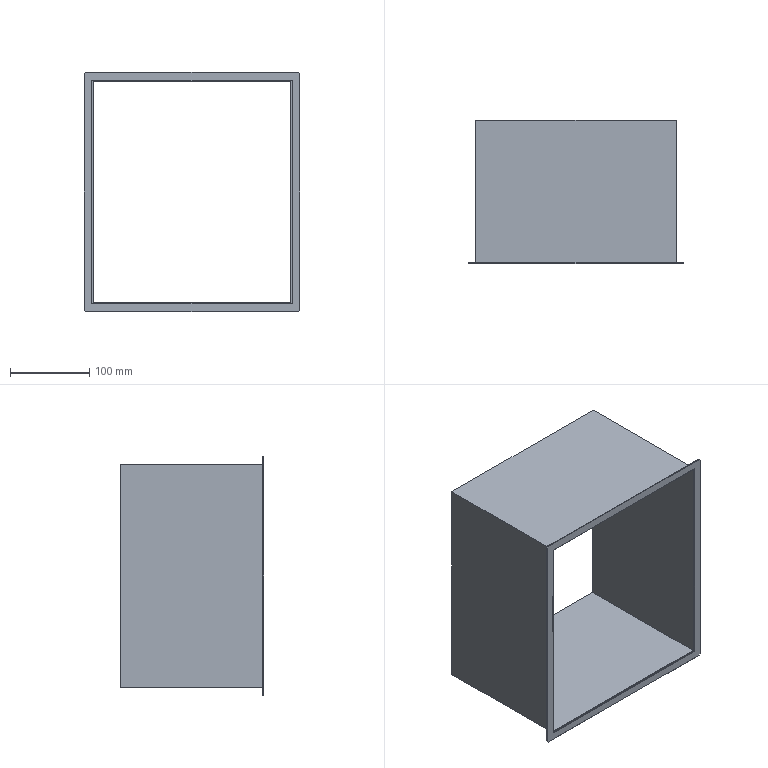Part | SolidWorks | features Chamfer 1, ExtruThin 1, ICE 1 | 2 solids | 24 faces | box 273 x 181.2 x 303 mm | volume 301154 mm3 | plane 24
STEP:
#1=CARTESIAN_POINT('',(126.5,180.,141.5));
#2=VERTEX_POINT('',#1);
#3=CARTESIAN_POINT('',(126.5,180.,-141.5));
#4=VERTEX_POINT('',#3);
#5=CARTESIAN_POINT('',(126.5,180.,0.));
#6=DIRECTION('',(0.,0.,-1.));
#7=VECTOR('',#6,1000.);
#8=LINE('',#5,#7);
#9=EDGE_CURVE('',#2,#4,#8,.T.);
#10=ORIENTED_EDGE('',*,*,#9,.T.);
#11=CARTESIAN_POINT('',(-126.5,180.,-141.5));
#12=VERTEX_POINT('',#11);
#13=CARTESIAN_POINT('',(0.,180.,-141.5));
#14=DIRECTION('',(-1.,0.,0.));
#15=VECTOR('',#14,1000.);
#16=LINE('',#13,#15);
#17=EDGE_CURVE('',#4,#12,#16,.T.);
#18=ORIENTED_EDGE('',*,*,#17,.T.);
#19=CARTESIAN_POINT('',(-126.5,180.,141.5));
#20=VERTEX_POINT('',#19);
#21=CARTESIAN_POINT('',(-126.5,180.,0.));
#22=DIRECTION('',(0.,0.,1.));
#23=VECTOR('',#22,1000.);
#24=LINE('',#21,#23);
#25=EDGE_CURVE('',#12,#20,#24,.T.);
#26=ORIENTED_EDGE('',*,*,#25,.T.);
#27=CARTESIAN_POINT('',(0.,180.,141.5));
#28=DIRECTION('',(1.,0.,0.));
#29=VECTOR('',#28,1000.);
#30=LINE('',#27,#29);
#31=EDGE_CURVE('',#20,#2,#30,.T.);
#32=ORIENTED_EDGE('',*,*,#31,.T.);
#33=EDGE_LOOP('',(#10,#18,#26,#32));
#34=FACE_OUTER_BOUND('',#33,.T.);
#35=CARTESIAN_POINT('',(125.,180.,-140.));
#36=VERTEX_POINT('',#35);
#37=CARTESIAN_POINT('',(-125.,180.,-140.));
#38=VERTEX_POINT('',#37);
#39=CARTESIAN_POINT('',(-125.,180.,-140.));
#40=DIRECTION('',(-1.,0.,0.));
#41=VECTOR('',#40,1000.);
#42=LINE('',#39,#41);
#43=EDGE_CURVE('',#36,#38,#42,.T.);
#44=ORIENTED_EDGE('',*,*,#43,.F.);
#45=CARTESIAN_POINT('',(125.,180.,140.));
#46=VERTEX_POINT('',#45);
#47=CARTESIAN_POINT('',(125.,180.,140.));
#48=DIRECTION('',(0.,0.,-1.));
#49=VECTOR('',#48,1000.);
#50=LINE('',#47,#49);
#51=EDGE_CURVE('',#46,#36,#50,.T.);
#52=ORIENTED_EDGE('',*,*,#51,.F.);
#53=CARTESIAN_POINT('',(-125.,180.,140.));
#54=VERTEX_POINT('',#53);
#55=CARTESIAN_POINT('',(-125.,180.,140.));
#56=DIRECTION('',(1.,0.,0.));
#57=VECTOR('',#56,1000.);
#58=LINE('',#55,#57);
#59=EDGE_CURVE('',#54,#46,#58,.T.);
#60=ORIENTED_EDGE('',*,*,#59,.F.);
#61=CARTESIAN_POINT('',(-125.,180.,140.));
#62=DIRECTION('',(0.,0.,1.));
#63=VECTOR('',#62,1000.);
#64=LINE('',#61,#63);
#65=EDGE_CURVE('',#38,#54,#64,.T.);
#66=ORIENTED_EDGE('',*,*,#65,.F.);
#67=EDGE_LOOP('',(#44,#52,#60,#66));
#68=FACE_BOUND('',#67,.T.);
#69=CARTESIAN_POINT('',(0.,180.,0.));
#70=DIRECTION('',(0.,1.,0.));
#71=DIRECTION('',(0.,0.,1.));
#72=AXIS2_PLACEMENT_3D('',#69,#70,#71);
#73=PLANE('',#72);
#74=ADVANCED_FACE('',(#34,#68),#73,.T.);
#75=CARTESIAN_POINT('',(126.5,0.,141.5));
#76=VERTEX_POINT('',#75);
#77=CARTESIAN_POINT('',(126.5,0.,-141.5));
#78=VERTEX_POINT('',#77);
#79=CARTESIAN_POINT('',(126.5,0.,0.));
#80=DIRECTION('',(0.,0.,-1.));
#81=VECTOR('',#80,1000.);
#82=LINE('',#79,#81);
#83=EDGE_CURVE('',#76,#78,#82,.T.);
#84=ORIENTED_EDGE('',*,*,#83,.F.);
#85=CARTESIAN_POINT('',(-126.5,0.,141.5));
#86=VERTEX_POINT('',#85);
#87=CARTESIAN_POINT('',(0.,0.,141.5));
#88=DIRECTION('',(1.,0.,0.));
#89=VECTOR('',#88,1000.);
#90=LINE('',#87,#89);
#91=EDGE_CURVE('',#86,#76,#90,.T.);
#92=ORIENTED_EDGE('',*,*,#91,.F.);
#93=CARTESIAN_POINT('',(-126.5,0.,-141.5));
#94=VERTEX_POINT('',#93);
#95=CARTESIAN_POINT('',(-126.5,0.,0.));
#96=DIRECTION('',(0.,0.,1.));
#97=VECTOR('',#96,1000.);
#98=LINE('',#95,#97);
#99=EDGE_CURVE('',#94,#86,#98,.T.);
#100=ORIENTED_EDGE('',*,*,#99,.F.);
#101=CARTESIAN_POINT('',(0.,0.,-141.5));
#102=DIRECTION('',(-1.,0.,0.));
#103=VECTOR('',#102,1000.);
#104=LINE('',#101,#103);
#105=EDGE_CURVE('',#78,#94,#104,.T.);
#106=ORIENTED_EDGE('',*,*,#105,.F.);
#107=EDGE_LOOP('',(#84,#92,#100,#106));
#108=FACE_OUTER_BOUND('',#107,.T.);
#109=CARTESIAN_POINT('',(125.,0.,140.));
#110=VERTEX_POINT('',#109);
#111=CARTESIAN_POINT('',(125.,0.,-140.));
#112=VERTEX_POINT('',#111);
#113=CARTESIAN_POINT('',(125.,0.,140.));
#114=DIRECTION('',(0.,0.,-1.));
#115=VECTOR('',#114,1000.);
#116=LINE('',#113,#115);
#117=EDGE_CURVE('',#110,#112,#116,.T.);
#118=ORIENTED_EDGE('',*,*,#117,.T.);
#119=CARTESIAN_POINT('',(-125.,0.,-140.));
#120=VERTEX_POINT('',#119);
#121=CARTESIAN_POINT('',(-125.,0.,-140.));
#122=DIRECTION('',(-1.,0.,0.));
#123=VECTOR('',#122,1000.);
#124=LINE('',#121,#123);
#125=EDGE_CURVE('',#112,#120,#124,.T.);
#126=ORIENTED_EDGE('',*,*,#125,.T.);
#127=CARTESIAN_POINT('',(-125.,0.,140.));
#128=VERTEX_POINT('',#127);
#129=CARTESIAN_POINT('',(-125.,0.,140.));
#130=DIRECTION('',(0.,0.,1.));
#131=VECTOR('',#130,1000.);
#132=LINE('',#129,#131);
#133=EDGE_CURVE('',#120,#128,#132,.T.);
#134=ORIENTED_EDGE('',*,*,#133,.T.);
#135=CARTESIAN_POINT('',(-125.,0.,140.));
#136=DIRECTION('',(1.,0.,0.));
#137=VECTOR('',#136,1000.);
#138=LINE('',#135,#137);
#139=EDGE_CURVE('',#128,#110,#138,.T.);
#140=ORIENTED_EDGE('',*,*,#139,.T.);
#141=EDGE_LOOP('',(#118,#126,#134,#140));
#142=FACE_BOUND('',#141,.T.);
#143=CARTESIAN_POINT('',(0.,0.,0.));
#144=DIRECTION('',(0.,1.,0.));
#145=DIRECTION('',(0.,0.,1.));
#146=AXIS2_PLACEMENT_3D('',#143,#144,#145);
#147=PLANE('',#146);
#148=ADVANCED_FACE('',(#108,#142),#147,.F.);
#149=ORIENTED_EDGE('',*,*,#83,.T.);
#150=CARTESIAN_POINT('',(126.5,180.,-141.5));
#151=DIRECTION('',(0.,-1.,0.));
#152=VECTOR('',#151,1000.);
#153=LINE('',#150,#152);
#154=EDGE_CURVE('',#4,#78,#153,.T.);
#155=ORIENTED_EDGE('',*,*,#154,.F.);
#156=ORIENTED_EDGE('',*,*,#9,.F.);
#157=CARTESIAN_POINT('',(126.5,180.,141.5));
#158=DIRECTION('',(0.,-1.,0.));
#159=VECTOR('',#158,1000.);
#160=LINE('',#157,#159);
#161=EDGE_CURVE('',#2,#76,#160,.T.);
#162=ORIENTED_EDGE('',*,*,#161,.T.);
#163=EDGE_LOOP('',(#149,#155,#156,#162));
#164=FACE_OUTER_BOUND('',#163,.T.);
#165=CARTESIAN_POINT('',(126.5,180.,0.));
#166=DIRECTION('',(-1.,0.,0.));
#167=DIRECTION('',(0.,0.,1.));
#168=AXIS2_PLACEMENT_3D('',#165,#166,#167);
#169=PLANE('',#168);
#170=ADVANCED_FACE('',(#164),#169,.F.);
#171=ORIENTED_EDGE('',*,*,#105,.T.);
#172=CARTESIAN_POINT('',(-126.5,180.,-141.5));
#173=DIRECTION('',(0.,-1.,0.));
#174=VECTOR('',#173,1000.);
#175=LINE('',#172,#174);
#176=EDGE_CURVE('',#12,#94,#175,.T.);
#177=ORIENTED_EDGE('',*,*,#176,.F.);
#178=ORIENTED_EDGE('',*,*,#17,.F.);
#179=ORIENTED_EDGE('',*,*,#154,.T.);
#180=EDGE_LOOP('',(#171,#177,#178,#179));
#181=FACE_OUTER_BOUND('',#180,.T.);
#182=CARTESIAN_POINT('',(0.,180.,-141.5));
#183=DIRECTION('',(0.,0.,1.));
#184=DIRECTION('',(1.,0.,0.));
#185=AXIS2_PLACEMENT_3D('',#182,#183,#184);
#186=PLANE('',#185);
#187=ADVANCED_FACE('',(#181),#186,.F.);
#188=ORIENTED_EDGE('',*,*,#99,.T.);
#189=CARTESIAN_POINT('',(-126.5,180.,141.5));
#190=DIRECTION('',(0.,-1.,0.));
#191=VECTOR('',#190,1000.);
#192=LINE('',#189,#191);
#193=EDGE_CURVE('',#20,#86,#192,.T.);
#194=ORIENTED_EDGE('',*,*,#193,.F.);
#195=ORIENTED_EDGE('',*,*,#25,.F.);
#196=ORIENTED_EDGE('',*,*,#176,.T.);
#197=EDGE_LOOP('',(#188,#194,#195,#196));
#198=FACE_OUTER_BOUND('',#197,.T.);
#199=CARTESIAN_POINT('',(-126.5,180.,0.));
#200=DIRECTION('',(1.,0.,0.));
#201=DIRECTION('',(0.,0.,-1.));
#202=AXIS2_PLACEMENT_3D('',#199,#200,#201);
#203=PLANE('',#202);
#204=ADVANCED_FACE('',(#198),#203,.F.);
#205=ORIENTED_EDGE('',*,*,#91,.T.);
#206=ORIENTED_EDGE('',*,*,#161,.F.);
#207=ORIENTED_EDGE('',*,*,#31,.F.);
#208=ORIENTED_EDGE('',*,*,#193,.T.);
#209=EDGE_LOOP('',(#205,#206,#207,#208));
#210=FACE_OUTER_BOUND('',#209,.T.);
#211=CARTESIAN_POINT('',(0.,180.,141.5));
#212=DIRECTION('',(0.,0.,-1.));
#213=DIRECTION('',(-1.,0.,0.));
#214=AXIS2_PLACEMENT_3D('',#211,#212,#213);
#215=PLANE('',#214);
#216=ADVANCED_FACE('',(#210),#215,.F.);
#217=ORIENTED_EDGE('',*,*,#117,.F.);
#218=CARTESIAN_POINT('',(125.,180.,140.));
#219=DIRECTION('',(0.,-1.,0.));
#220=VECTOR('',#219,1000.);
#221=LINE('',#218,#220);
#222=EDGE_CURVE('',#46,#110,#221,.T.);
#223=ORIENTED_EDGE('',*,*,#222,.F.);
#224=ORIENTED_EDGE('',*,*,#51,.T.);
#225=CARTESIAN_POINT('',(125.,180.,-140.));
#226=DIRECTION('',(0.,-1.,0.));
#227=VECTOR('',#226,1000.);
#228=LINE('',#225,#227);
#229=EDGE_CURVE('',#36,#112,#228,.T.);
#230=ORIENTED_EDGE('',*,*,#229,.T.);
#231=EDGE_LOOP('',(#217,#223,#224,#230));
#232=FACE_OUTER_BOUND('',#231,.T.);
#233=CARTESIAN_POINT('',(125.,180.,140.));
#234=DIRECTION('',(-1.,0.,0.));
#235=DIRECTION('',(0.,0.,1.));
#236=AXIS2_PLACEMENT_3D('',#233,#234,#235);
#237=PLANE('',#236);
#238=ADVANCED_FACE('',(#232),#237,.T.);
#239=ORIENTED_EDGE('',*,*,#125,.F.);
#240=ORIENTED_EDGE('',*,*,#229,.F.);
#241=ORIENTED_EDGE('',*,*,#43,.T.);
#242=CARTESIAN_POINT('',(-125.,180.,-140.));
#243=DIRECTION('',(0.,-1.,0.));
#244=VECTOR('',#243,1000.);
#245=LINE('',#242,#244);
#246=EDGE_CURVE('',#38,#120,#245,.T.);
#247=ORIENTED_EDGE('',*,*,#246,.T.);
#248=EDGE_LOOP('',(#239,#240,#241,#247));
#249=FACE_OUTER_BOUND('',#248,.T.);
#250=CARTESIAN_POINT('',(-125.,180.,-140.));
#251=DIRECTION('',(0.,0.,1.));
#252=DIRECTION('',(1.,0.,0.));
#253=AXIS2_PLACEMENT_3D('',#250,#251,#252);
#254=PLANE('',#253);
#255=ADVANCED_FACE('',(#249),#254,.T.);
#256=ORIENTED_EDGE('',*,*,#133,.F.);
#257=ORIENTED_EDGE('',*,*,#246,.F.);
#258=ORIENTED_EDGE('',*,*,#65,.T.);
#259=CARTESIAN_POINT('',(-125.,180.,140.));
#260=DIRECTION('',(0.,-1.,0.));
#261=VECTOR('',#260,1000.);
#262=LINE('',#259,#261);
#263=EDGE_CURVE('',#54,#128,#262,.T.);
#264=ORIENTED_EDGE('',*,*,#263,.T.);
#265=EDGE_LOOP('',(#256,#257,#258,#264));
#266=FACE_OUTER_BOUND('',#265,.T.);
#267=CARTESIAN_POINT('',(-125.,180.,140.));
#268=DIRECTION('',(1.,0.,0.));
#269=DIRECTION('',(0.,0.,-1.));
#270=AXIS2_PLACEMENT_3D('',#267,#268,#269);
#271=PLANE('',#270);
#272=ADVANCED_FACE('',(#266),#271,.T.);
#273=ORIENTED_EDGE('',*,*,#139,.F.);
#274=ORIENTED_EDGE('',*,*,#263,.F.);
#275=ORIENTED_EDGE('',*,*,#59,.T.);
#276=ORIENTED_EDGE('',*,*,#222,.T.);
#277=EDGE_LOOP('',(#273,#274,#275,#276));
#278=FACE_OUTER_BOUND('',#277,.T.);
#279=CARTESIAN_POINT('',(-125.,180.,140.));
#280=DIRECTION('',(0.,0.,-1.));
#281=DIRECTION('',(-1.,0.,0.));
#282=AXIS2_PLACEMENT_3D('',#279,#280,#281);
#283=PLANE('',#282);
#284=ADVANCED_FACE('',(#278),#283,.T.);
#285=CLOSED_SHELL('',(#74,#148,#170,#187,#204,#216,#238,#255,#272,#284));
#286=MANIFOLD_SOLID_BREP('',#285);
#287=CARTESIAN_POINT('',(134.5,-1.2,151.5));
#288=VERTEX_POINT('',#287);
#289=CARTESIAN_POINT('',(-134.5,-1.2,151.5));
#290=VERTEX_POINT('',#289);
#291=CARTESIAN_POINT('',(136.5,-1.2,151.5));
#292=DIRECTION('',(-1.,0.,0.));
#293=VECTOR('',#292,1000.);
#294=LINE('',#291,#293);
#295=EDGE_CURVE('',#288,#290,#294,.T.);
#296=ORIENTED_EDGE('',*,*,#295,.T.);
#297=CARTESIAN_POINT('',(-136.5,-1.2,149.5));
#298=VERTEX_POINT('',#297);
#299=CARTESIAN_POINT('',(-143.,-1.2,143.));
#300=DIRECTION('',(-0.7071,0.,-0.7071));
#301=VECTOR('',#300,1000.);
#302=LINE('',#299,#301);
#303=EDGE_CURVE('',#290,#298,#302,.T.);
#304=ORIENTED_EDGE('',*,*,#303,.T.);
#305=CARTESIAN_POINT('',(-136.5,-1.2,-149.5));
#306=VERTEX_POINT('',#305);
#307=CARTESIAN_POINT('',(-136.5,-1.2,151.5));
#308=DIRECTION('',(0.,0.,-1.));
#309=VECTOR('',#308,1000.);
#310=LINE('',#307,#309);
#311=EDGE_CURVE('',#298,#306,#310,.T.);
#312=ORIENTED_EDGE('',*,*,#311,.T.);
#313=CARTESIAN_POINT('',(-134.5,-1.2,-151.5));
#314=VERTEX_POINT('',#313);
#315=CARTESIAN_POINT('',(-143.,-1.2,-143.));
#316=DIRECTION('',(0.7071,0.,-0.7071));
#317=VECTOR('',#316,1000.);
#318=LINE('',#315,#317);
#319=EDGE_CURVE('',#306,#314,#318,.T.);
#320=ORIENTED_EDGE('',*,*,#319,.T.);
#321=CARTESIAN_POINT('',(134.5,-1.2,-151.5));
#322=VERTEX_POINT('',#321);
#323=CARTESIAN_POINT('',(-136.5,-1.2,-151.5));
#324=DIRECTION('',(1.,0.,0.));
#325=VECTOR('',#324,1000.);
#326=LINE('',#323,#325);
#327=EDGE_CURVE('',#314,#322,#326,.T.);
#328=ORIENTED_EDGE('',*,*,#327,.T.);
#329=CARTESIAN_POINT('',(136.5,-1.2,-149.5));
#330=VERTEX_POINT('',#329);
#331=CARTESIAN_POINT('',(143.,-1.2,-143.));
#332=DIRECTION('',(0.7071,0.,0.7071));
#333=VECTOR('',#332,1000.);
#334=LINE('',#331,#333);
#335=EDGE_CURVE('',#322,#330,#334,.T.);
#336=ORIENTED_EDGE('',*,*,#335,.T.);
#337=CARTESIAN_POINT('',(136.5,-1.2,149.5));
#338=VERTEX_POINT('',#337);
#339=CARTESIAN_POINT('',(136.5,-1.2,-151.5));
#340=DIRECTION('',(0.,0.,1.));
#341=VECTOR('',#340,1000.);
#342=LINE('',#339,#341);
#343=EDGE_CURVE('',#330,#338,#342,.T.);
#344=ORIENTED_EDGE('',*,*,#343,.T.);
#345=CARTESIAN_POINT('',(143.,-1.2,143.));
#346=DIRECTION('',(-0.7071,0.,0.7071));
#347=VECTOR('',#346,1000.);
#348=LINE('',#345,#347);
#349=EDGE_CURVE('',#338,#288,#348,.T.);
#350=ORIENTED_EDGE('',*,*,#349,.T.);
#351=EDGE_LOOP('',(#296,#304,#312,#320,#328,#336,#344,#350));
#352=FACE_OUTER_BOUND('',#351,.T.);
#353=CARTESIAN_POINT('',(-126.5,-1.2,-141.5));
#354=VERTEX_POINT('',#353);
#355=CARTESIAN_POINT('',(126.5,-1.2,-141.5));
#356=VERTEX_POINT('',#355);
#357=CARTESIAN_POINT('',(-126.5,-1.2,-141.5));
#358=DIRECTION('',(1.,0.,0.));
#359=VECTOR('',#358,1000.);
#360=LINE('',#357,#359);
#361=EDGE_CURVE('',#354,#356,#360,.T.);
#362=ORIENTED_EDGE('',*,*,#361,.F.);
#363=CARTESIAN_POINT('',(-126.5,-1.2,141.5));
#364=VERTEX_POINT('',#363);
#365=CARTESIAN_POINT('',(-126.5,-1.2,141.5));
#366=DIRECTION('',(0.,0.,-1.));
#367=VECTOR('',#366,1000.);
#368=LINE('',#365,#367);
#369=EDGE_CURVE('',#364,#354,#368,.T.);
#370=ORIENTED_EDGE('',*,*,#369,.F.);
#371=CARTESIAN_POINT('',(126.5,-1.2,141.5));
#372=VERTEX_POINT('',#371);
#373=CARTESIAN_POINT('',(-126.5,-1.2,141.5));
#374=DIRECTION('',(-1.,0.,0.));
#375=VECTOR('',#374,1000.);
#376=LINE('',#373,#375);
#377=EDGE_CURVE('',#372,#364,#376,.T.);
#378=ORIENTED_EDGE('',*,*,#377,.F.);
#379=CARTESIAN_POINT('',(126.5,-1.2,141.5));
#380=DIRECTION('',(0.,0.,1.));
#381=VECTOR('',#380,1000.);
#382=LINE('',#379,#381);
#383=EDGE_CURVE('',#356,#372,#382,.T.);
#384=ORIENTED_EDGE('',*,*,#383,.F.);
#385=EDGE_LOOP('',(#362,#370,#378,#384));
#386=FACE_BOUND('',#385,.T.);
#387=CARTESIAN_POINT('',(0.,-1.2,0.));
#388=DIRECTION('',(0.,-1.,0.));
#389=DIRECTION('',(0.,0.,-1.));
#390=AXIS2_PLACEMENT_3D('',#387,#388,#389);
#391=PLANE('',#390);
#392=ADVANCED_FACE('',(#352,#386),#391,.T.);
#393=CARTESIAN_POINT('',(-136.5,0.,149.5));
#394=VERTEX_POINT('',#393);
#395=CARTESIAN_POINT('',(-136.5,0.,-149.5));
#396=VERTEX_POINT('',#395);
#397=CARTESIAN_POINT('',(-136.5,0.,151.5));
#398=DIRECTION('',(0.,0.,-1.));
#399=VECTOR('',#398,1000.);
#400=LINE('',#397,#399);
#401=EDGE_CURVE('',#394,#396,#400,.T.);
#402=ORIENTED_EDGE('',*,*,#401,.F.);
#403=CARTESIAN_POINT('',(-134.5,0.,151.5));
#404=VERTEX_POINT('',#403);
#405=CARTESIAN_POINT('',(-136.5,0.,149.5));
#406=DIRECTION('',(0.7071,0.,0.7071));
#407=VECTOR('',#406,1000.);
#408=LINE('',#405,#407);
#409=EDGE_CURVE('',#394,#404,#408,.T.);
#410=ORIENTED_EDGE('',*,*,#409,.T.);
#411=CARTESIAN_POINT('',(134.5,0.,151.5));
#412=VERTEX_POINT('',#411);
#413=CARTESIAN_POINT('',(136.5,0.,151.5));
#414=DIRECTION('',(-1.,0.,0.));
#415=VECTOR('',#414,1000.);
#416=LINE('',#413,#415);
#417=EDGE_CURVE('',#412,#404,#416,.T.);
#418=ORIENTED_EDGE('',*,*,#417,.F.);
#419=CARTESIAN_POINT('',(136.5,0.,149.5));
#420=VERTEX_POINT('',#419);
#421=CARTESIAN_POINT('',(134.5,0.,151.5));
#422=DIRECTION('',(0.7071,0.,-0.7071));
#423=VECTOR('',#422,1000.);
#424=LINE('',#421,#423);
#425=EDGE_CURVE('',#412,#420,#424,.T.);
#426=ORIENTED_EDGE('',*,*,#425,.T.);
#427=CARTESIAN_POINT('',(136.5,0.,-149.5));
#428=VERTEX_POINT('',#427);
#429=CARTESIAN_POINT('',(136.5,0.,-151.5));
#430=DIRECTION('',(0.,0.,1.));
#431=VECTOR('',#430,1000.);
#432=LINE('',#429,#431);
#433=EDGE_CURVE('',#428,#420,#432,.T.);
#434=ORIENTED_EDGE('',*,*,#433,.F.);
#435=CARTESIAN_POINT('',(134.5,0.,-151.5));
#436=VERTEX_POINT('',#435);
#437=CARTESIAN_POINT('',(136.5,0.,-149.5));
#438=DIRECTION('',(-0.7071,0.,-0.7071));
#439=VECTOR('',#438,1000.);
#440=LINE('',#437,#439);
#441=EDGE_CURVE('',#428,#436,#440,.T.);
#442=ORIENTED_EDGE('',*,*,#441,.T.);
#443=CARTESIAN_POINT('',(-134.5,0.,-151.5));
#444=VERTEX_POINT('',#443);
#445=CARTESIAN_POINT('',(-136.5,0.,-151.5));
#446=DIRECTION('',(1.,0.,0.));
#447=VECTOR('',#446,1000.);
#448=LINE('',#445,#447);
#449=EDGE_CURVE('',#444,#436,#448,.T.);
#450=ORIENTED_EDGE('',*,*,#449,.F.);
#451=CARTESIAN_POINT('',(-134.5,0.,-151.5));
#452=DIRECTION('',(-0.7071,0.,0.7071));
#453=VECTOR('',#452,1000.);
#454=LINE('',#451,#453);
#455=EDGE_CURVE('',#444,#396,#454,.T.);
#456=ORIENTED_EDGE('',*,*,#455,.T.);
#457=EDGE_LOOP('',(#402,#410,#418,#426,#434,#442,#450,#456));
#458=FACE_OUTER_BOUND('',#457,.T.);
#459=CARTESIAN_POINT('',(-126.5,0.,141.5));
#460=VERTEX_POINT('',#459);
#461=CARTESIAN_POINT('',(-126.5,0.,-141.5));
#462=VERTEX_POINT('',#461);
#463=CARTESIAN_POINT('',(-126.5,0.,141.5));
#464=DIRECTION('',(0.,0.,-1.));
#465=VECTOR('',#464,1000.);
#466=LINE('',#463,#465);
#467=EDGE_CURVE('',#460,#462,#466,.T.);
#468=ORIENTED_EDGE('',*,*,#467,.T.);
#469=CARTESIAN_POINT('',(126.5,0.,-141.5));
#470=VERTEX_POINT('',#469);
#471=CARTESIAN_POINT('',(-126.5,0.,-141.5));
#472=DIRECTION('',(1.,0.,0.));
#473=VECTOR('',#472,1000.);
#474=LINE('',#471,#473);
#475=EDGE_CURVE('',#462,#470,#474,.T.);
#476=ORIENTED_EDGE('',*,*,#475,.T.);
#477=CARTESIAN_POINT('',(126.5,0.,141.5));
#478=VERTEX_POINT('',#477);
#479=CARTESIAN_POINT('',(126.5,0.,141.5));
#480=DIRECTION('',(0.,0.,1.));
#481=VECTOR('',#480,1000.);
#482=LINE('',#479,#481);
#483=EDGE_CURVE('',#470,#478,#482,.T.);
#484=ORIENTED_EDGE('',*,*,#483,.T.);
#485=CARTESIAN_POINT('',(-126.5,0.,141.5));
#486=DIRECTION('',(-1.,0.,0.));
#487=VECTOR('',#486,1000.);
#488=LINE('',#485,#487);
#489=EDGE_CURVE('',#478,#460,#488,.T.);
#490=ORIENTED_EDGE('',*,*,#489,.T.);
#491=EDGE_LOOP('',(#468,#476,#484,#490));
#492=FACE_BOUND('',#491,.T.);
#493=CARTESIAN_POINT('',(0.,0.,0.));
#494=DIRECTION('',(0.,-1.,0.));
#495=DIRECTION('',(0.,0.,-1.));
#496=AXIS2_PLACEMENT_3D('',#493,#494,#495);
#497=PLANE('',#496);
#498=ADVANCED_FACE('',(#458,#492),#497,.F.);
#499=ORIENTED_EDGE('',*,*,#327,.F.);
#500=CARTESIAN_POINT('',(-134.5,-1.2,-151.5));
#501=DIRECTION('',(0.,1.,0.));
#502=VECTOR('',#501,1000.);
#503=LINE('',#500,#502);
#504=EDGE_CURVE('',#314,#444,#503,.T.);
#505=ORIENTED_EDGE('',*,*,#504,.T.);
#506=ORIENTED_EDGE('',*,*,#449,.T.);
#507=CARTESIAN_POINT('',(134.5,-1.2,-151.5));
#508=DIRECTION('',(0.,-1.,0.));
#509=VECTOR('',#508,1000.);
#510=LINE('',#507,#509);
#511=EDGE_CURVE('',#436,#322,#510,.T.);
#512=ORIENTED_EDGE('',*,*,#511,.T.);
#513=EDGE_LOOP('',(#499,#505,#506,#512));
#514=FACE_OUTER_BOUND('',#513,.T.);
#515=CARTESIAN_POINT('',(-136.5,-1.2,-151.5));
#516=DIRECTION('',(0.,0.,1.));
#517=DIRECTION('',(1.,0.,0.));
#518=AXIS2_PLACEMENT_3D('',#515,#516,#517);
#519=PLANE('',#518);
#520=ADVANCED_FACE('',(#514),#519,.F.);
#521=ORIENTED_EDGE('',*,*,#343,.F.);
#522=CARTESIAN_POINT('',(136.5,-1.2,-149.5));
#523=DIRECTION('',(0.,1.,0.));
#524=VECTOR('',#523,1000.);
#525=LINE('',#522,#524);
#526=EDGE_CURVE('',#330,#428,#525,.T.);
#527=ORIENTED_EDGE('',*,*,#526,.T.);
#528=ORIENTED_EDGE('',*,*,#433,.T.);
#529=CARTESIAN_POINT('',(136.5,-1.2,149.5));
#530=DIRECTION('',(0.,-1.,0.));
#531=VECTOR('',#530,1000.);
#532=LINE('',#529,#531);
#533=EDGE_CURVE('',#420,#338,#532,.T.);
#534=ORIENTED_EDGE('',*,*,#533,.T.);
#535=EDGE_LOOP('',(#521,#527,#528,#534));
#536=FACE_OUTER_BOUND('',#535,.T.);
#537=CARTESIAN_POINT('',(136.5,-1.2,-151.5));
#538=DIRECTION('',(-1.,0.,0.));
#539=DIRECTION('',(0.,0.,1.));
#540=AXIS2_PLACEMENT_3D('',#537,#538,#539);
#541=PLANE('',#540);
#542=ADVANCED_FACE('',(#536),#541,.F.);
#543=ORIENTED_EDGE('',*,*,#417,.T.);
#544=CARTESIAN_POINT('',(-134.5,-1.2,151.5));
#545=DIRECTION('',(0.,-1.,0.));
#546=VECTOR('',#545,1000.);
#547=LINE('',#544,#546);
#548=EDGE_CURVE('',#404,#290,#547,.T.);
#549=ORIENTED_EDGE('',*,*,#548,.T.);
#550=ORIENTED_EDGE('',*,*,#295,.F.);
#551=CARTESIAN_POINT('',(134.5,-1.2,151.5));
#552=DIRECTION('',(0.,1.,0.));
#553=VECTOR('',#552,1000.);
#554=LINE('',#551,#553);
#555=EDGE_CURVE('',#288,#412,#554,.T.);
#556=ORIENTED_EDGE('',*,*,#555,.T.);
#557=EDGE_LOOP('',(#543,#549,#550,#556));
#558=FACE_OUTER_BOUND('',#557,.T.);
#559=CARTESIAN_POINT('',(136.5,-1.2,151.5));
#560=DIRECTION('',(0.,0.,-1.));
#561=DIRECTION('',(-1.,0.,0.));
#562=AXIS2_PLACEMENT_3D('',#559,#560,#561);
#563=PLANE('',#562);
#564=ADVANCED_FACE('',(#558),#563,.F.);
#565=ORIENTED_EDGE('',*,*,#311,.F.);
#566=CARTESIAN_POINT('',(-136.5,-1.2,149.5));
#567=DIRECTION('',(0.,1.,0.));
#568=VECTOR('',#567,1000.);
#569=LINE('',#566,#568);
#570=EDGE_CURVE('',#298,#394,#569,.T.);
#571=ORIENTED_EDGE('',*,*,#570,.T.);
#572=ORIENTED_EDGE('',*,*,#401,.T.);
#573=CARTESIAN_POINT('',(-136.5,-1.2,-149.5));
#574=DIRECTION('',(0.,-1.,0.));
#575=VECTOR('',#574,1000.);
#576=LINE('',#573,#575);
#577=EDGE_CURVE('',#396,#306,#576,.T.);
#578=ORIENTED_EDGE('',*,*,#577,.T.);
#579=EDGE_LOOP('',(#565,#571,#572,#578));
#580=FACE_OUTER_BOUND('',#579,.T.);
#581=CARTESIAN_POINT('',(-136.5,-1.2,151.5));
#582=DIRECTION('',(1.,0.,0.));
#583=DIRECTION('',(0.,0.,-1.));
#584=AXIS2_PLACEMENT_3D('',#581,#582,#583);
#585=PLANE('',#584);
#586=ADVANCED_FACE('',(#580),#585,.F.);
#587=ORIENTED_EDGE('',*,*,#467,.F.);
#588=CARTESIAN_POINT('',(-126.5,-1.2,141.5));
#589=DIRECTION('',(0.,1.,0.));
#590=VECTOR('',#589,1000.);
#591=LINE('',#588,#590);
#592=EDGE_CURVE('',#364,#460,#591,.T.);
#593=ORIENTED_EDGE('',*,*,#592,.F.);
#594=ORIENTED_EDGE('',*,*,#369,.T.);
#595=CARTESIAN_POINT('',(-126.5,-1.2,-141.5));
#596=DIRECTION('',(0.,1.,0.));
#597=VECTOR('',#596,1000.);
#598=LINE('',#595,#597);
#599=EDGE_CURVE('',#354,#462,#598,.T.);
#600=ORIENTED_EDGE('',*,*,#599,.T.);
#601=EDGE_LOOP('',(#587,#593,#594,#600));
#602=FACE_OUTER_BOUND('',#601,.T.);
#603=CARTESIAN_POINT('',(-126.5,-1.2,141.5));
#604=DIRECTION('',(1.,0.,0.));
#605=DIRECTION('',(0.,0.,-1.));
#606=AXIS2_PLACEMENT_3D('',#603,#604,#605);
#607=PLANE('',#606);
#608=ADVANCED_FACE('',(#602),#607,.T.);
#609=ORIENTED_EDGE('',*,*,#475,.F.);
#610=ORIENTED_EDGE('',*,*,#599,.F.);
#611=ORIENTED_EDGE('',*,*,#361,.T.);
#612=CARTESIAN_POINT('',(126.5,-1.2,-141.5));
#613=DIRECTION('',(0.,1.,0.));
#614=VECTOR('',#613,1000.);
#615=LINE('',#612,#614);
#616=EDGE_CURVE('',#356,#470,#615,.T.);
#617=ORIENTED_EDGE('',*,*,#616,.T.);
#618=EDGE_LOOP('',(#609,#610,#611,#617));
#619=FACE_OUTER_BOUND('',#618,.T.);
#620=CARTESIAN_POINT('',(-126.5,-1.2,-141.5));
#621=DIRECTION('',(0.,0.,1.));
#622=DIRECTION('',(1.,0.,0.));
#623=AXIS2_PLACEMENT_3D('',#620,#621,#622);
#624=PLANE('',#623);
#625=ADVANCED_FACE('',(#619),#624,.T.);
#626=ORIENTED_EDGE('',*,*,#483,.F.);
#627=ORIENTED_EDGE('',*,*,#616,.F.);
#628=ORIENTED_EDGE('',*,*,#383,.T.);
#629=CARTESIAN_POINT('',(126.5,-1.2,141.5));
#630=DIRECTION('',(0.,1.,0.));
#631=VECTOR('',#630,1000.);
#632=LINE('',#629,#631);
#633=EDGE_CURVE('',#372,#478,#632,.T.);
#634=ORIENTED_EDGE('',*,*,#633,.T.);
#635=EDGE_LOOP('',(#626,#627,#628,#634));
#636=FACE_OUTER_BOUND('',#635,.T.);
#637=CARTESIAN_POINT('',(126.5,-1.2,141.5));
#638=DIRECTION('',(-1.,0.,0.));
#639=DIRECTION('',(0.,0.,1.));
#640=AXIS2_PLACEMENT_3D('',#637,#638,#639);
#641=PLANE('',#640);
#642=ADVANCED_FACE('',(#636),#641,.T.);
#643=ORIENTED_EDGE('',*,*,#489,.F.);
#644=ORIENTED_EDGE('',*,*,#633,.F.);
#645=ORIENTED_EDGE('',*,*,#377,.T.);
#646=ORIENTED_EDGE('',*,*,#592,.T.);
#647=EDGE_LOOP('',(#643,#644,#645,#646));
#648=FACE_OUTER_BOUND('',#647,.T.);
#649=CARTESIAN_POINT('',(-126.5,-1.2,141.5));
#650=DIRECTION('',(0.,0.,-1.));
#651=DIRECTION('',(-1.,0.,0.));
#652=AXIS2_PLACEMENT_3D('',#649,#650,#651);
#653=PLANE('',#652);
#654=ADVANCED_FACE('',(#648),#653,.T.);
#655=ORIENTED_EDGE('',*,*,#303,.F.);
#656=ORIENTED_EDGE('',*,*,#548,.F.);
#657=ORIENTED_EDGE('',*,*,#409,.F.);
#658=ORIENTED_EDGE('',*,*,#570,.F.);
#659=EDGE_LOOP('',(#655,#656,#657,#658));
#660=FACE_OUTER_BOUND('',#659,.T.);
#661=CARTESIAN_POINT('',(-136.5,-1.2,149.5));
#662=DIRECTION('',(0.7071,0.,-0.7071));
#663=DIRECTION('',(0.,1.,0.));
#664=AXIS2_PLACEMENT_3D('',#661,#662,#663);
#665=PLANE('',#664);
#666=ADVANCED_FACE('',(#660),#665,.F.);
#667=ORIENTED_EDGE('',*,*,#319,.F.);
#668=ORIENTED_EDGE('',*,*,#577,.F.);
#669=ORIENTED_EDGE('',*,*,#455,.F.);
#670=ORIENTED_EDGE('',*,*,#504,.F.);
#671=EDGE_LOOP('',(#667,#668,#669,#670));
#672=FACE_OUTER_BOUND('',#671,.T.);
#673=CARTESIAN_POINT('',(-134.5,-1.2,-151.5));
#674=DIRECTION('',(0.7071,0.,0.7071));
#675=DIRECTION('',(0.,1.,0.));
#676=AXIS2_PLACEMENT_3D('',#673,#674,#675);
#677=PLANE('',#676);
#678=ADVANCED_FACE('',(#672),#677,.F.);
#679=ORIENTED_EDGE('',*,*,#335,.F.);
#680=ORIENTED_EDGE('',*,*,#511,.F.);
#681=ORIENTED_EDGE('',*,*,#441,.F.);
#682=ORIENTED_EDGE('',*,*,#526,.F.);
#683=EDGE_LOOP('',(#679,#680,#681,#682));
#684=FACE_OUTER_BOUND('',#683,.T.);
#685=CARTESIAN_POINT('',(136.5,-1.2,-149.5));
#686=DIRECTION('',(-0.7071,0.,0.7071));
#687=DIRECTION('',(0.,1.,0.));
#688=AXIS2_PLACEMENT_3D('',#685,#686,#687);
#689=PLANE('',#688);
#690=ADVANCED_FACE('',(#684),#689,.F.);
#691=ORIENTED_EDGE('',*,*,#349,.F.);
#692=ORIENTED_EDGE('',*,*,#533,.F.);
#693=ORIENTED_EDGE('',*,*,#425,.F.);
#694=ORIENTED_EDGE('',*,*,#555,.F.);
#695=EDGE_LOOP('',(#691,#692,#693,#694));
#696=FACE_OUTER_BOUND('',#695,.T.);
#697=CARTESIAN_POINT('',(134.5,-1.2,151.5));
#698=DIRECTION('',(-0.7071,0.,-0.7071));
#699=DIRECTION('',(0.,1.,0.));
#700=AXIS2_PLACEMENT_3D('',#697,#698,#699);
#701=PLANE('',#700);
#702=ADVANCED_FACE('',(#696),#701,.F.);
#703=CLOSED_SHELL('',(#392,#498,#520,#542,#564,#586,#608,#625,#642,#654,#666,#678,#690,#702));
#704=MANIFOLD_SOLID_BREP('',#703);
#705=CARTESIAN_POINT('',(0.,0.,0.));
#706=DIRECTION('',(0.,0.,1.));
#707=DIRECTION('',(1.,0.,0.));
#708=AXIS2_PLACEMENT_3D('',#705,#706,#707);
#709=(LENGTH_UNIT()NAMED_UNIT(*)SI_UNIT(.MILLI.,.METRE.));
#710=UNCERTAINTY_MEASURE_WITH_UNIT(LENGTH_MEASURE(0.00001),#709,'','');
#711=(NAMED_UNIT(*)PLANE_ANGLE_UNIT()SI_UNIT($,.RADIAN.));
#712=(NAMED_UNIT(*)SI_UNIT($,.STERADIAN.)SOLID_ANGLE_UNIT());
#713=(GEOMETRIC_REPRESENTATION_CONTEXT(3)GLOBAL_UNCERTAINTY_ASSIGNED_CONTEXT((#710))GLOBAL_UNIT_ASSIGNED_CONTEXT((#709,#711,#712))REPRESENTATION_CONTEXT('',''));
#714=ADVANCED_BREP_SHAPE_REPRESENTATION('',(#286,#704,#708),#713);